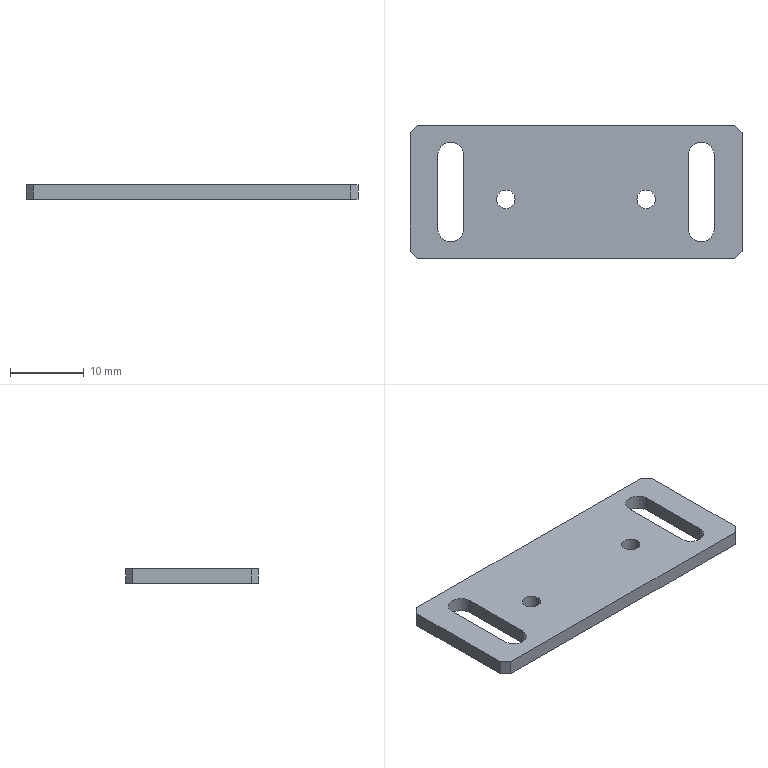Part | STEP file | PN_0107 Mount electronic clip sensor 5 | 1 solid | 22 faces | box 45 x 18 x 2 mm | volume 1418 mm3 | plane 14 | cylinder 8 | commonest cylinder face diameters 2.5 x4 3.5 x4